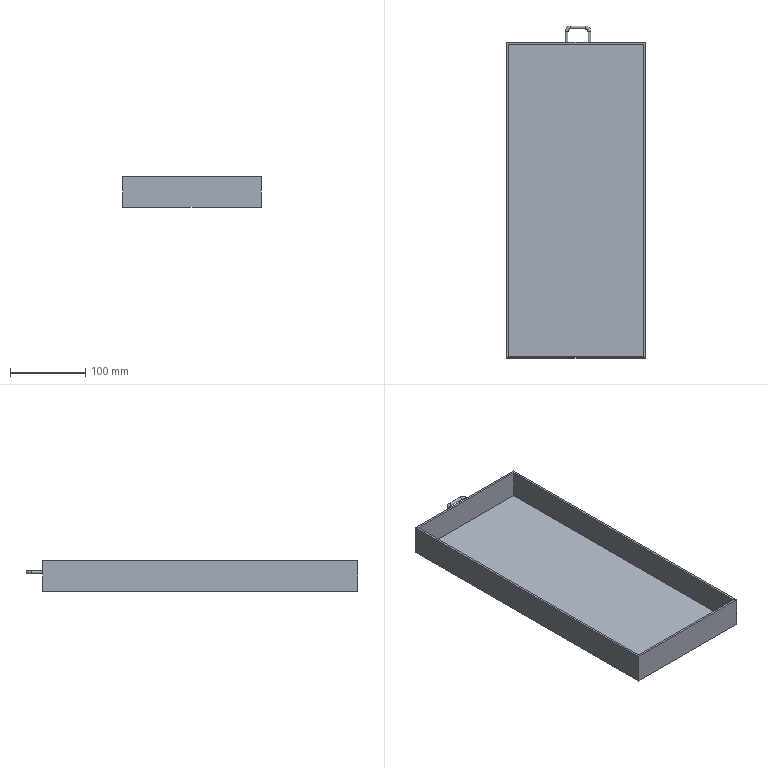Part | NX | features solid 2 | 1 solid | 16 faces | box 185 x 442 x 40 mm | volume 307576 mm3 | plane 11 | cylinder 3 | torus 2 | commonest cylinder face diameters 4 x3
STEP:
#1=CARTESIAN_POINT('',(-410.,375.,-368.));
#2=VERTEX_POINT('',#1);
#3=CARTESIAN_POINT('',(-410.,375.,-370.));
#4=DIRECTION('',(0.,1.,0.));
#5=DIRECTION('',(0.,0.,1.));
#6=AXIS2_PLACEMENT_3D('',#3,#4,#5);
#7=CIRCLE('',#6,2.);
#8=EDGE_CURVE('',#2,#2,#7,.T.);
#9=ORIENTED_EDGE('',*,*,#8,.F.);
#10=EDGE_LOOP('',(#9));
#11=FACE_BOUND('',#10,.T.);
#12=CARTESIAN_POINT('',(-490.,375.,-395.));
#13=VERTEX_POINT('',#12);
#14=CARTESIAN_POINT('',(-305.,375.,-395.));
#15=VERTEX_POINT('',#14);
#16=CARTESIAN_POINT('',(-450.,375.,-395.));
#17=DIRECTION('',(1.,0.,0.));
#18=VECTOR('',#17,1000.);
#19=LINE('',#16,#18);
#20=EDGE_CURVE('',#13,#15,#19,.T.);
#21=ORIENTED_EDGE('',*,*,#20,.F.);
#22=CARTESIAN_POINT('',(-490.,375.,-355.));
#23=VERTEX_POINT('',#22);
#24=CARTESIAN_POINT('',(-490.,375.,-345.));
#25=DIRECTION('',(0.,0.,-1.));
#26=VECTOR('',#25,1000.);
#27=LINE('',#24,#26);
#28=EDGE_CURVE('',#23,#13,#27,.T.);
#29=ORIENTED_EDGE('',*,*,#28,.F.);
#30=CARTESIAN_POINT('',(-305.,375.,-355.));
#31=VERTEX_POINT('',#30);
#32=CARTESIAN_POINT('',(-300.,375.,-355.));
#33=DIRECTION('',(1.,0.,0.));
#34=VECTOR('',#33,1000.);
#35=LINE('',#32,#34);
#36=EDGE_CURVE('',#23,#31,#35,.T.);
#37=ORIENTED_EDGE('',*,*,#36,.T.);
#38=CARTESIAN_POINT('',(-305.,375.,-345.));
#39=DIRECTION('',(0.,0.,-1.));
#40=VECTOR('',#39,1000.);
#41=LINE('',#38,#40);
#42=EDGE_CURVE('',#31,#15,#41,.T.);
#43=ORIENTED_EDGE('',*,*,#42,.T.);
#44=EDGE_LOOP('',(#21,#29,#37,#43));
#45=FACE_BOUND('',#44,.T.);
#46=CARTESIAN_POINT('',(-380.,375.,-368.));
#47=VERTEX_POINT('',#46);
#48=CARTESIAN_POINT('',(-380.,375.,-370.));
#49=DIRECTION('',(0.,1.,0.));
#50=DIRECTION('',(0.,0.,1.));
#51=AXIS2_PLACEMENT_3D('',#48,#49,#50);
#52=CIRCLE('',#51,2.);
#53=EDGE_CURVE('',#47,#47,#52,.T.);
#54=ORIENTED_EDGE('',*,*,#53,.F.);
#55=EDGE_LOOP('',(#54));
#56=FACE_BOUND('',#55,.T.);
#57=CARTESIAN_POINT('',(-450.,375.,-345.));
#58=DIRECTION('',(0.,1.,0.));
#59=DIRECTION('',(0.,0.,1.));
#60=AXIS2_PLACEMENT_3D('',#57,#58,#59);
#61=PLANE('',#60);
#62=ADVANCED_FACE('',(#11,#45,#56),#61,.T.);
#63=CARTESIAN_POINT('',(-307.5,372.5,-392.5));
#64=VERTEX_POINT('',#63);
#65=CARTESIAN_POINT('',(-307.5,-42.5,-392.5));
#66=VERTEX_POINT('',#65);
#67=CARTESIAN_POINT('',(-307.5,182.5,-392.5));
#68=DIRECTION('',(0.,-1.,0.));
#69=VECTOR('',#68,1000.);
#70=LINE('',#67,#69);
#71=EDGE_CURVE('',#64,#66,#70,.T.);
#72=ORIENTED_EDGE('',*,*,#71,.F.);
#73=CARTESIAN_POINT('',(-487.5,372.5,-392.5));
#74=VERTEX_POINT('',#73);
#75=CARTESIAN_POINT('',(-447.5,372.5,-392.5));
#76=DIRECTION('',(1.,0.,0.));
#77=VECTOR('',#76,1000.);
#78=LINE('',#75,#77);
#79=EDGE_CURVE('',#74,#64,#78,.T.);
#80=ORIENTED_EDGE('',*,*,#79,.F.);
#81=CARTESIAN_POINT('',(-487.5,-42.5,-392.5));
#82=VERTEX_POINT('',#81);
#83=CARTESIAN_POINT('',(-487.5,372.5,-392.5));
#84=DIRECTION('',(0.,1.,0.));
#85=VECTOR('',#84,1000.);
#86=LINE('',#83,#85);
#87=EDGE_CURVE('',#82,#74,#86,.T.);
#88=ORIENTED_EDGE('',*,*,#87,.F.);
#89=CARTESIAN_POINT('',(-450.,-42.5,-392.5));
#90=DIRECTION('',(-1.,0.,0.));
#91=VECTOR('',#90,1000.);
#92=LINE('',#89,#91);
#93=EDGE_CURVE('',#66,#82,#92,.T.);
#94=ORIENTED_EDGE('',*,*,#93,.F.);
#95=EDGE_LOOP('',(#72,#80,#88,#94));
#96=FACE_BOUND('',#95,.T.);
#97=CARTESIAN_POINT('',(-302.5,182.5,-392.5));
#98=DIRECTION('',(0.,0.,-1.));
#99=DIRECTION('',(-1.,0.,0.));
#100=AXIS2_PLACEMENT_3D('',#97,#98,#99);
#101=PLANE('',#100);
#102=ADVANCED_FACE('',(#96),#101,.F.);
#103=CARTESIAN_POINT('',(-305.,-45.,-395.));
#104=VERTEX_POINT('',#103);
#105=CARTESIAN_POINT('',(-490.,-45.,-395.));
#106=VERTEX_POINT('',#105);
#107=CARTESIAN_POINT('',(-302.5,-45.,-395.));
#108=DIRECTION('',(-1.,0.,0.));
#109=VECTOR('',#108,1000.);
#110=LINE('',#107,#109);
#111=EDGE_CURVE('',#104,#106,#110,.T.);
#112=ORIENTED_EDGE('',*,*,#111,.T.);
#113=CARTESIAN_POINT('',(-490.,182.5,-395.));
#114=DIRECTION('',(0.,1.,0.));
#115=VECTOR('',#114,1000.);
#116=LINE('',#113,#115);
#117=EDGE_CURVE('',#106,#13,#116,.T.);
#118=ORIENTED_EDGE('',*,*,#117,.T.);
#119=ORIENTED_EDGE('',*,*,#20,.T.);
#120=CARTESIAN_POINT('',(-305.,182.5,-395.));
#121=DIRECTION('',(0.,-1.,0.));
#122=VECTOR('',#121,1000.);
#123=LINE('',#120,#122);
#124=EDGE_CURVE('',#15,#104,#123,.T.);
#125=ORIENTED_EDGE('',*,*,#124,.T.);
#126=EDGE_LOOP('',(#112,#118,#119,#125));
#127=FACE_BOUND('',#126,.T.);
#128=CARTESIAN_POINT('',(-302.5,182.5,-395.));
#129=DIRECTION('',(0.,0.,-1.));
#130=DIRECTION('',(-1.,0.,0.));
#131=AXIS2_PLACEMENT_3D('',#128,#129,#130);
#132=PLANE('',#131);
#133=ADVANCED_FACE('',(#127),#132,.T.);
#134=CARTESIAN_POINT('',(-307.5,372.5,-355.));
#135=VERTEX_POINT('',#134);
#136=CARTESIAN_POINT('',(-307.5,372.5,-345.));
#137=DIRECTION('',(0.,0.,-1.));
#138=VECTOR('',#137,1000.);
#139=LINE('',#136,#138);
#140=EDGE_CURVE('',#135,#64,#139,.T.);
#141=ORIENTED_EDGE('',*,*,#140,.F.);
#142=CARTESIAN_POINT('',(-487.5,372.5,-355.));
#143=VERTEX_POINT('',#142);
#144=CARTESIAN_POINT('',(-300.,372.5,-355.));
#145=DIRECTION('',(-1.,0.,0.));
#146=VECTOR('',#145,1000.);
#147=LINE('',#144,#146);
#148=EDGE_CURVE('',#135,#143,#147,.T.);
#149=ORIENTED_EDGE('',*,*,#148,.T.);
#150=CARTESIAN_POINT('',(-487.5,372.5,-345.));
#151=DIRECTION('',(0.,0.,-1.));
#152=VECTOR('',#151,1000.);
#153=LINE('',#150,#152);
#154=EDGE_CURVE('',#143,#74,#153,.T.);
#155=ORIENTED_EDGE('',*,*,#154,.T.);
#156=ORIENTED_EDGE('',*,*,#79,.T.);
#157=EDGE_LOOP('',(#141,#149,#155,#156));
#158=FACE_BOUND('',#157,.T.);
#159=CARTESIAN_POINT('',(-300.,372.5,-345.));
#160=DIRECTION('',(0.,-1.,0.));
#161=DIRECTION('',(0.,0.,-1.));
#162=AXIS2_PLACEMENT_3D('',#159,#160,#161);
#163=PLANE('',#162);
#164=ADVANCED_FACE('',(#158),#163,.T.);
#165=ORIENTED_EDGE('',*,*,#124,.F.);
#166=ORIENTED_EDGE('',*,*,#42,.F.);
#167=CARTESIAN_POINT('',(-305.,-45.,-355.));
#168=VERTEX_POINT('',#167);
#169=CARTESIAN_POINT('',(-305.,372.5,-355.));
#170=DIRECTION('',(0.,-1.,0.));
#171=VECTOR('',#170,1000.);
#172=LINE('',#169,#171);
#173=EDGE_CURVE('',#31,#168,#172,.T.);
#174=ORIENTED_EDGE('',*,*,#173,.T.);
#175=CARTESIAN_POINT('',(-305.,-45.,-345.));
#176=DIRECTION('',(0.,0.,-1.));
#177=VECTOR('',#176,1000.);
#178=LINE('',#175,#177);
#179=EDGE_CURVE('',#168,#104,#178,.T.);
#180=ORIENTED_EDGE('',*,*,#179,.T.);
#181=EDGE_LOOP('',(#165,#166,#174,#180));
#182=FACE_BOUND('',#181,.T.);
#183=CARTESIAN_POINT('',(-305.,375.,-345.));
#184=DIRECTION('',(1.,0.,0.));
#185=DIRECTION('',(0.,0.,-1.));
#186=AXIS2_PLACEMENT_3D('',#183,#184,#185);
#187=PLANE('',#186);
#188=ADVANCED_FACE('',(#182),#187,.T.);
#189=ORIENTED_EDGE('',*,*,#117,.F.);
#190=CARTESIAN_POINT('',(-490.,-45.,-355.));
#191=VERTEX_POINT('',#190);
#192=CARTESIAN_POINT('',(-490.,-45.,-345.));
#193=DIRECTION('',(0.,0.,-1.));
#194=VECTOR('',#193,1000.);
#195=LINE('',#192,#194);
#196=EDGE_CURVE('',#191,#106,#195,.T.);
#197=ORIENTED_EDGE('',*,*,#196,.F.);
#198=CARTESIAN_POINT('',(-490.,372.5,-355.));
#199=DIRECTION('',(0.,1.,0.));
#200=VECTOR('',#199,1000.);
#201=LINE('',#198,#200);
#202=EDGE_CURVE('',#191,#23,#201,.T.);
#203=ORIENTED_EDGE('',*,*,#202,.T.);
#204=ORIENTED_EDGE('',*,*,#28,.T.);
#205=EDGE_LOOP('',(#189,#197,#203,#204));
#206=FACE_BOUND('',#205,.T.);
#207=CARTESIAN_POINT('',(-490.,372.5,-345.));
#208=DIRECTION('',(-1.,0.,0.));
#209=DIRECTION('',(0.,0.,1.));
#210=AXIS2_PLACEMENT_3D('',#207,#208,#209);
#211=PLANE('',#210);
#212=ADVANCED_FACE('',(#206),#211,.T.);
#213=ORIENTED_EDGE('',*,*,#148,.F.);
#214=CARTESIAN_POINT('',(-307.5,-42.5,-355.));
#215=VERTEX_POINT('',#214);
#216=CARTESIAN_POINT('',(-307.5,372.5,-355.));
#217=DIRECTION('',(0.,1.,0.));
#218=VECTOR('',#217,1000.);
#219=LINE('',#216,#218);
#220=EDGE_CURVE('',#215,#135,#219,.T.);
#221=ORIENTED_EDGE('',*,*,#220,.F.);
#222=CARTESIAN_POINT('',(-487.5,-42.5,-355.));
#223=VERTEX_POINT('',#222);
#224=CARTESIAN_POINT('',(-300.,-42.5,-355.));
#225=DIRECTION('',(1.,0.,0.));
#226=VECTOR('',#225,1000.);
#227=LINE('',#224,#226);
#228=EDGE_CURVE('',#223,#215,#227,.T.);
#229=ORIENTED_EDGE('',*,*,#228,.F.);
#230=CARTESIAN_POINT('',(-487.5,372.5,-355.));
#231=DIRECTION('',(0.,-1.,0.));
#232=VECTOR('',#231,1000.);
#233=LINE('',#230,#232);
#234=EDGE_CURVE('',#143,#223,#233,.T.);
#235=ORIENTED_EDGE('',*,*,#234,.F.);
#236=EDGE_LOOP('',(#213,#221,#229,#235));
#237=FACE_BOUND('',#236,.T.);
#238=ORIENTED_EDGE('',*,*,#173,.F.);
#239=ORIENTED_EDGE('',*,*,#36,.F.);
#240=ORIENTED_EDGE('',*,*,#202,.F.);
#241=CARTESIAN_POINT('',(-300.,-45.,-355.));
#242=DIRECTION('',(-1.,0.,0.));
#243=VECTOR('',#242,1000.);
#244=LINE('',#241,#243);
#245=EDGE_CURVE('',#168,#191,#244,.T.);
#246=ORIENTED_EDGE('',*,*,#245,.F.);
#247=EDGE_LOOP('',(#238,#239,#240,#246));
#248=FACE_BOUND('',#247,.T.);
#249=CARTESIAN_POINT('',(-300.,372.5,-355.));
#250=DIRECTION('',(0.,0.,-1.));
#251=DIRECTION('',(-1.,0.,0.));
#252=AXIS2_PLACEMENT_3D('',#249,#250,#251);
#253=PLANE('',#252);
#254=ADVANCED_FACE('',(#237,#248),#253,.F.);
#255=CARTESIAN_POINT('',(-307.5,-42.5,-345.));
#256=DIRECTION('',(0.,0.,-1.));
#257=VECTOR('',#256,1000.);
#258=LINE('',#255,#257);
#259=EDGE_CURVE('',#215,#66,#258,.T.);
#260=ORIENTED_EDGE('',*,*,#259,.T.);
#261=ORIENTED_EDGE('',*,*,#93,.T.);
#262=CARTESIAN_POINT('',(-487.5,-42.5,-345.));
#263=DIRECTION('',(0.,0.,-1.));
#264=VECTOR('',#263,1000.);
#265=LINE('',#262,#264);
#266=EDGE_CURVE('',#223,#82,#265,.T.);
#267=ORIENTED_EDGE('',*,*,#266,.F.);
#268=ORIENTED_EDGE('',*,*,#228,.T.);
#269=EDGE_LOOP('',(#260,#261,#267,#268));
#270=FACE_BOUND('',#269,.T.);
#271=CARTESIAN_POINT('',(-450.,-42.5,-345.));
#272=DIRECTION('',(0.,1.,0.));
#273=DIRECTION('',(0.,0.,1.));
#274=AXIS2_PLACEMENT_3D('',#271,#272,#273);
#275=PLANE('',#274);
#276=ADVANCED_FACE('',(#270),#275,.T.);
#277=ORIENTED_EDGE('',*,*,#111,.F.);
#278=ORIENTED_EDGE('',*,*,#179,.F.);
#279=ORIENTED_EDGE('',*,*,#245,.T.);
#280=ORIENTED_EDGE('',*,*,#196,.T.);
#281=EDGE_LOOP('',(#277,#278,#279,#280));
#282=FACE_BOUND('',#281,.T.);
#283=CARTESIAN_POINT('',(-300.,-45.,-345.));
#284=DIRECTION('',(0.,-1.,0.));
#285=DIRECTION('',(0.,0.,-1.));
#286=AXIS2_PLACEMENT_3D('',#283,#284,#285);
#287=PLANE('',#286);
#288=ADVANCED_FACE('',(#282),#287,.T.);
#289=ORIENTED_EDGE('',*,*,#87,.T.);
#290=ORIENTED_EDGE('',*,*,#154,.F.);
#291=ORIENTED_EDGE('',*,*,#234,.T.);
#292=ORIENTED_EDGE('',*,*,#266,.T.);
#293=EDGE_LOOP('',(#289,#290,#291,#292));
#294=FACE_BOUND('',#293,.T.);
#295=CARTESIAN_POINT('',(-487.5,372.5,-345.));
#296=DIRECTION('',(1.,0.,0.));
#297=DIRECTION('',(0.,0.,-1.));
#298=AXIS2_PLACEMENT_3D('',#295,#296,#297);
#299=PLANE('',#298);
#300=ADVANCED_FACE('',(#294),#299,.T.);
#301=ORIENTED_EDGE('',*,*,#71,.T.);
#302=ORIENTED_EDGE('',*,*,#259,.F.);
#303=ORIENTED_EDGE('',*,*,#220,.T.);
#304=ORIENTED_EDGE('',*,*,#140,.T.);
#305=EDGE_LOOP('',(#301,#302,#303,#304));
#306=FACE_BOUND('',#305,.T.);
#307=CARTESIAN_POINT('',(-307.5,182.5,-345.));
#308=DIRECTION('',(-1.,0.,0.));
#309=DIRECTION('',(0.,0.,1.));
#310=AXIS2_PLACEMENT_3D('',#307,#308,#309);
#311=PLANE('',#310);
#312=ADVANCED_FACE('',(#306),#311,.T.);
#313=CARTESIAN_POINT('',(-410.,390.,-368.));
#314=VERTEX_POINT('',#313);
#315=CARTESIAN_POINT('',(-410.,390.,-370.));
#316=DIRECTION('',(0.,-1.,0.));
#317=DIRECTION('',(0.,0.,1.));
#318=AXIS2_PLACEMENT_3D('',#315,#316,#317);
#319=CIRCLE('',#318,2.);
#320=EDGE_CURVE('',#314,#314,#319,.T.);
#321=ORIENTED_EDGE('',*,*,#320,.T.);
#322=EDGE_LOOP('',(#321));
#323=FACE_BOUND('',#322,.T.);
#324=ORIENTED_EDGE('',*,*,#8,.T.);
#325=EDGE_LOOP('',(#324));
#326=FACE_BOUND('',#325,.T.);
#327=CARTESIAN_POINT('',(-410.,390.,-370.));
#328=DIRECTION('',(0.,-1.,0.));
#329=DIRECTION('',(0.,0.,-1.));
#330=AXIS2_PLACEMENT_3D('',#327,#328,#329);
#331=CYLINDRICAL_SURFACE('',#330,2.);
#332=ADVANCED_FACE('',(#323,#326),#331,.T.);
#333=CARTESIAN_POINT('',(-405.,395.,-368.));
#334=VERTEX_POINT('',#333);
#335=CARTESIAN_POINT('',(-405.,395.,-370.));
#336=DIRECTION('',(-1.,0.,0.));
#337=DIRECTION('',(0.,0.,1.));
#338=AXIS2_PLACEMENT_3D('',#335,#336,#337);
#339=CIRCLE('',#338,2.);
#340=EDGE_CURVE('',#334,#334,#339,.T.);
#341=ORIENTED_EDGE('',*,*,#340,.T.);
#342=EDGE_LOOP('',(#341));
#343=FACE_BOUND('',#342,.T.);
#344=ORIENTED_EDGE('',*,*,#320,.F.);
#345=EDGE_LOOP('',(#344));
#346=FACE_BOUND('',#345,.T.);
#347=CARTESIAN_POINT('',(-405.,390.,-370.));
#348=DIRECTION('',(0.,0.,1.));
#349=DIRECTION('',(1.,0.,0.));
#350=AXIS2_PLACEMENT_3D('',#347,#348,#349);
#351=TOROIDAL_SURFACE('',#350,5.,2.);
#352=ADVANCED_FACE('',(#343,#346),#351,.T.);
#353=CARTESIAN_POINT('',(-385.,395.,-368.));
#354=VERTEX_POINT('',#353);
#355=CARTESIAN_POINT('',(-385.,395.,-370.));
#356=DIRECTION('',(-1.,0.,0.));
#357=DIRECTION('',(0.,0.,1.));
#358=AXIS2_PLACEMENT_3D('',#355,#356,#357);
#359=CIRCLE('',#358,2.);
#360=EDGE_CURVE('',#354,#354,#359,.T.);
#361=ORIENTED_EDGE('',*,*,#360,.T.);
#362=EDGE_LOOP('',(#361));
#363=FACE_BOUND('',#362,.T.);
#364=ORIENTED_EDGE('',*,*,#340,.F.);
#365=EDGE_LOOP('',(#364));
#366=FACE_BOUND('',#365,.T.);
#367=CARTESIAN_POINT('',(-385.,395.,-370.));
#368=DIRECTION('',(-1.,0.,0.));
#369=DIRECTION('',(0.,0.,1.));
#370=AXIS2_PLACEMENT_3D('',#367,#368,#369);
#371=CYLINDRICAL_SURFACE('',#370,2.);
#372=ADVANCED_FACE('',(#363,#366),#371,.T.);
#373=CARTESIAN_POINT('',(-380.,390.,-368.));
#374=VERTEX_POINT('',#373);
#375=CARTESIAN_POINT('',(-380.,390.,-370.));
#376=DIRECTION('',(0.,1.,0.));
#377=DIRECTION('',(0.,0.,1.));
#378=AXIS2_PLACEMENT_3D('',#375,#376,#377);
#379=CIRCLE('',#378,2.);
#380=EDGE_CURVE('',#374,#374,#379,.T.);
#381=ORIENTED_EDGE('',*,*,#380,.T.);
#382=EDGE_LOOP('',(#381));
#383=FACE_BOUND('',#382,.T.);
#384=ORIENTED_EDGE('',*,*,#360,.F.);
#385=EDGE_LOOP('',(#384));
#386=FACE_BOUND('',#385,.T.);
#387=CARTESIAN_POINT('',(-385.,390.,-370.));
#388=DIRECTION('',(0.,0.,1.));
#389=DIRECTION('',(1.,0.,0.));
#390=AXIS2_PLACEMENT_3D('',#387,#388,#389);
#391=TOROIDAL_SURFACE('',#390,5.,2.);
#392=ADVANCED_FACE('',(#383,#386),#391,.T.);
#393=ORIENTED_EDGE('',*,*,#380,.F.);
#394=EDGE_LOOP('',(#393));
#395=FACE_BOUND('',#394,.T.);
#396=ORIENTED_EDGE('',*,*,#53,.T.);
#397=EDGE_LOOP('',(#396));
#398=FACE_BOUND('',#397,.T.);
#399=CARTESIAN_POINT('',(-380.,390.,-370.));
#400=DIRECTION('',(0.,-1.,0.));
#401=DIRECTION('',(0.,0.,-1.));
#402=AXIS2_PLACEMENT_3D('',#399,#400,#401);
#403=CYLINDRICAL_SURFACE('',#402,2.);
#404=ADVANCED_FACE('',(#395,#398),#403,.T.);
#405=CLOSED_SHELL('',(#62,#102,#133,#164,#188,#212,#254,#276,#288,#300,#312,#332,#352,#372,#392,#404));
#406=MANIFOLD_SOLID_BREP('',#405);
#407=(LENGTH_UNIT()NAMED_UNIT(*)SI_UNIT(.MILLI.,.METRE.));
#408=UNCERTAINTY_MEASURE_WITH_UNIT(LENGTH_MEASURE(0.00001),#407,'','');
#409=(NAMED_UNIT(*)PLANE_ANGLE_UNIT()SI_UNIT($,.RADIAN.));
#410=(NAMED_UNIT(*)SI_UNIT($,.STERADIAN.)SOLID_ANGLE_UNIT());
#411=(GEOMETRIC_REPRESENTATION_CONTEXT(3)GLOBAL_UNCERTAINTY_ASSIGNED_CONTEXT((#408))GLOBAL_UNIT_ASSIGNED_CONTEXT((#407,#409,#410))REPRESENTATION_CONTEXT('',''));
#412=ADVANCED_BREP_SHAPE_REPRESENTATION('',(#406),#411);